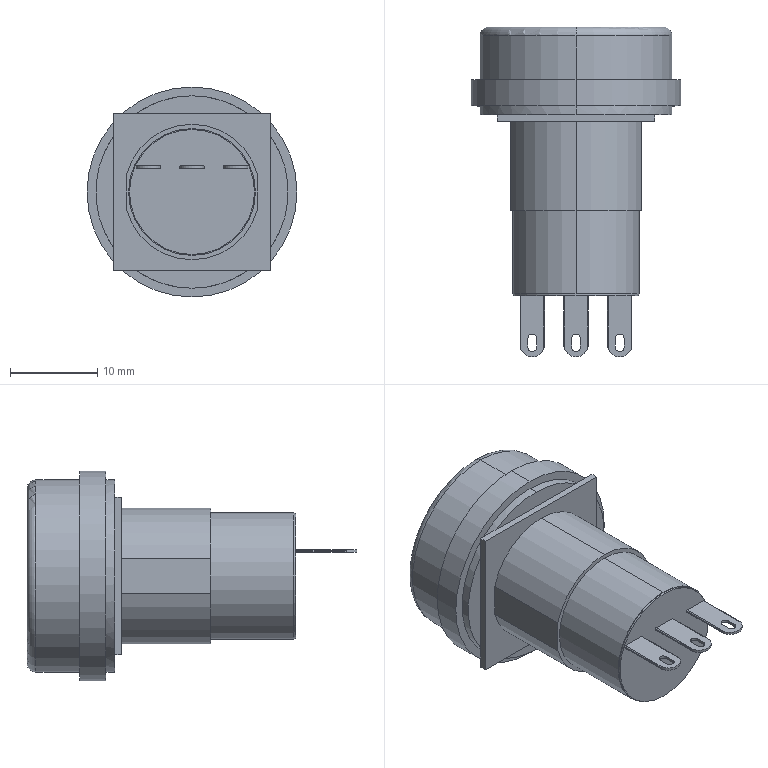Part | STEP file | Indicator light AD17-22-AC220VW white | 1 solid | 75 faces | box 24 x 37.7 x 24 mm | volume 7790 mm3 | plane 39 | cylinder 34 | torus 2 | commonest cylinder face diameters 0.2 x12 1 x6 22 x4 2.8 x3 15.5 x3 14.3 x2